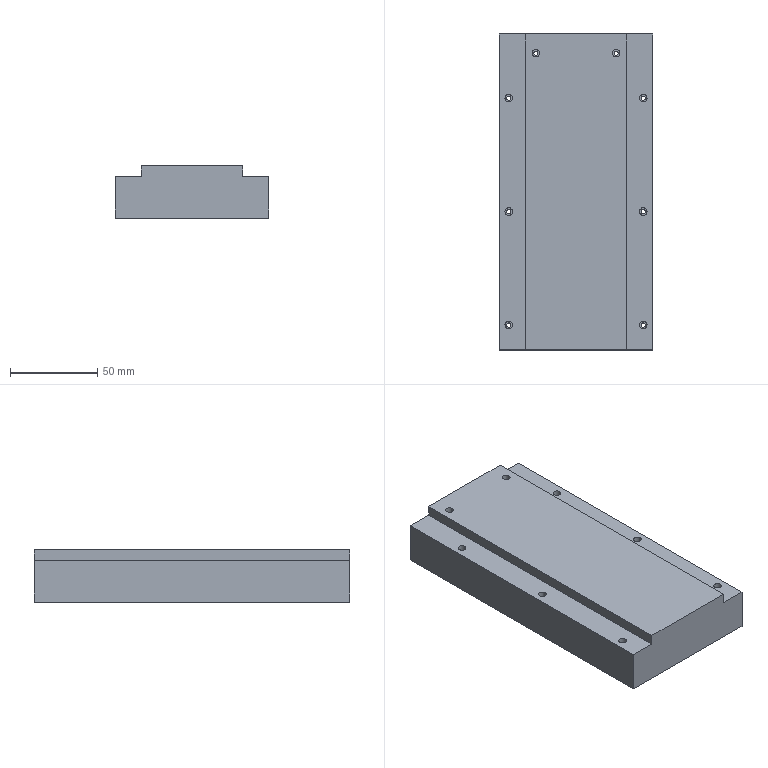NC program | NX | posted with a generic post | part box 88 x 181.05 x 30 mm
Lines 5542 to 5691 of 14572:
(PLANAR_MILL_9_COPY_1_COPY , TOOL : D12-36-D12-120-3T-FINISH)
N11046 T03 M6
N11048 G54
N11050 G17 G43 G0 G90 X-50.265 Y19.409 B0. C296.438 S4500 H3 M3
N11052 Z32.5
N11054 Z5.5
N11056 G94 G1 Z2.5 F800.
N11058 X-39.52 Y14.066
N11060 X35.067 Y-23.021
N11062 X45.812 Y-28.363
N11064 Z5.5
N11066 G0 Z32.5
(PLANAR_MILL_10_COPY_1 , TOOL : D12-36-D12-120-3T-FINISH)
N11068 G3P2 X0. Y0. Z0. I90. J12.8666 K-83.5258
N11070 G53.1
N11072 X-120.624 Y19.704 Z29.988 H3
N11074 Z2.988
N11076 G1 Z-0.012
N11078 X-103.412 Y17.751
N11080 X-104.605 Y11.871
N11082 X-106.624 Y-5.923
N11084 X-25.84 Y-31.878
N11086 X-18.04 Y36.858
N11088 X-102.586 Y29.664
N11090 X-104.605 Y11.871
N11092 X-98.643 Y11.194
N11094 X-109.374 Y12.412
N11096 X-111.837 Y-9.289
N11098 X-21.731 Y-38.24
N11100 X-12.61 Y42.137
N11102 X-106.912 Y34.113
N11104 X-109.374 Y12.412
N11106 X-103.413 Y11.735
N11108 Z2.988
N11110 G0 Z29.988
(PLANAR_MILL_13_COPY , TOOL : D12-36-D12-120-3T-FINISH)
N11112 X-22.769 Y-47.384
N11114 Z1.988
N11116 G1 Z-0.012
N11118 X-21.867 Y-39.435
N11120 X-12.474 Y43.332
N11122 X-11.572 Y51.281
N11124 Z1.988
N11126 G0 Z29.988
N11128 G69
(FLOOR_WALL_COPY_COPY , TOOL : D12-36-D12-120-3T-FINISH)
N11130 G3P2 X0. Y0. Z0. I-90. J7.5 K86.2419
N11132 G53.1
N11134 X-126.992 Y-42.408 Z71.298 H3
N11136 Z41.298
N11138 G1 Z38.298
N11140 X-128.626 Y-33.558
N11142 G3 X-132.121 Y-31.152 R3.
N11144 G1 X-163.688 Y-36.981
N11146 X-167.119 Y15.252
N11148 X-107.228 Y12.171
N11150 X-104.714 Y-26.092
N11152 X-132.121 Y-31.152
N11154 X-133.755 Y-22.302
N11156 X-155.371 Y-26.293
N11158 X-157.475 Y5.744
N11160 X-115.684 Y3.594
N11162 X-114.22 Y-18.695
N11164 X-133.755 Y-22.302
N11166 X-135.389 Y-13.451
N11168 X-147.054 Y-15.605
N11170 X-147.831 Y-3.764
N11172 X-124.14 Y-4.983
N11174 X-123.725 Y-11.298
N11176 X-135.389 Y-13.451
N11178 X-136.373 Y-13.633
N11180 G3 X-138.778 Y-17.128 R3.
N11182 G1 Z41.298
N11184 G0 Z71.298
N11186 G69
(PLANAR_MILL_12_COPY_COPY , TOOL : D12-36-D12-120-3T-FINISH)
N11188 G3P2 X0. Y0. Z0. I-90. J65. K50.4263
N11190 G53.1
N11192 X-80.941 Y1.741 Z192.908 H3
N11194 Z165.908
N11196 G1 Z162.908
N11198 X-73.296 Y-7.508
N11200 X-21.174 Y-70.572
N11202 X-13.53 Y-79.821
N11204 Z165.908
N11206 G0 Z192.908
N11208 X-86.491 Y-2.846
N11210 Z165.908
N11212 G1 Z162.908
N11214 X-78.846 Y-12.095
N11216 X-26.724 Y-75.159
N11218 X-19.079 Y-84.408
N11220 Z165.908
N11222 G0 Z192.908
N11224 G69
(FLOOR_WALL_2_COPY_2 , TOOL : D12-36-D12-120-3T-FINISH)
N11226 G3P2 X0. Y0. Z0. I0. J48. K63.562
N11228 G53.1
N11230 X-17.735 Y-18.87 Z65.624 H3
N11232 Z35.674
N11234 G1 Z32.674
N11236 X-19.071 Y-16.184
N11238 X-103.813 Y154.245
N11240 X-95.74 Y155.283
N11242 X-24.306 Y11.621
N11244 X-28.561 Y37.452
N11246 X-87.666 Y156.321
N11248 X-81.084 Y157.167
N11250 X-76.239 Y150.616
N11252 X-32.815 Y63.284
N11254 X-31.479 Y60.598
N11256 X-29.389 Y60.942
N11258 Z35.674
N11260 G0 Z65.624
N11262 G69
(FLOOR_WALL_2_COPY_1_COPY_COPY , TOOL : D12-36-D12-120-3T-FINISH)
N11264 G3P2 X0. Y0. Z0. I180. J48. K63.562
N11266 G53.1
N11268 X35.072 Y-64.656 Z65.624 H3
N11270 Z35.624
N11272 G1 Z32.624
N11274 X33.536 Y-66.115
N11276 X34.872 Y-68.801
N11278 X71.165 Y-141.791
N11280 X76.376 Y-159.508
N11282 X73.063 Y-162.885
N11284 X16.843 Y-49.819
N11286 X-1.185 Y-30.836
N11288 X67.363 Y-168.696
N11290 X61.663 Y-174.507
N11292 X-22.802 Y-4.637
N11294 X-24.138 Y-1.951
N11296 Z35.624
N11298 G0 Z65.624
N11300 G69
N11302 M5